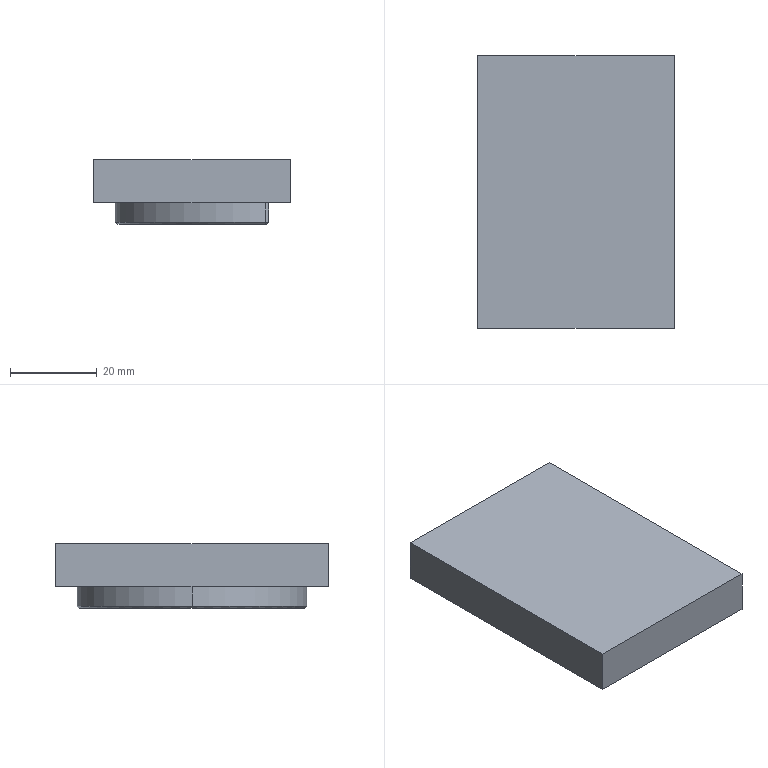NC program | NX | posted with a generic post | part box 45.394 x 63 x 15 mm
Whole program:
N10 G17 G21 G94 G90
(FLOOR_WALL_COPY , TOOL : D80)
N12 T19 M6
N14 G54
N16 G17 G0 G90 X71.5 Y0. S5000 M3
N18 G43 Z30. H19
N20 Z7.
N22 G94 G1 Z4. F1200.
N24 X66.5
N26 X-66.5
N28 X-71.5
N30 Z7.
N32 G0 Z30.
N34 X71.5
N36 Z6.
N38 G1 Z3.
N40 X66.5
N42 X-66.5
N44 X-71.5
N46 Z6.
N48 G0 Z30.
N50 X71.5
N52 Z5.
N54 G1 Z2.
N56 X66.5
N58 X-66.5
N60 X-71.5
N62 Z5.
N64 G0 Z30.
N66 X71.5
N68 Z4.
N70 G1 Z1.
N72 X66.5
N74 X-66.5
N76 X-71.5
N78 Z4.
N80 G0 Z30.
N82 X71.5
N84 Z3.
N86 G1 Z0.
N88 X66.5
N90 X-66.5
N92 X-71.5
N94 Z3.
N96 G0 Z30.
N98 M5
(HOLE_MILLING_1 , TOOL : D2)
N100 T17 M6
N102 G54
N104 G17 G0 G90 X0. Y13.197 S9500 M3
N106 G43 Z30. H17
N108 Z0.5
N110 G94 G3 X-0.253 Y12.945 R0.253 F1050.
N112 X0. Y12.692 R0.253
N114 X0. Y12.692 Z0.35 I0. J0.505
N116 X0. Y12.692 Z0.2 I0. J0.505
N118 X0. Y12.692 Z0.05 I0. J0.505
N120 X0. Y12.692 Z-0.1 I0. J0.505
N122 X0. Y12.692 Z-0.25 I0. J0.505
N124 X0. Y12.692 Z-0.4 I0. J0.505
N126 X0. Y12.692 Z-0.55 I0. J0.505
N128 X0. Y12.692 Z-0.7 I0. J0.505
N130 X0. Y12.692 Z-0.85 I0. J0.505
N132 X0. Y12.692 Z-1. I0. J0.505
N134 X0. Y12.692 Z-1.15 I0. J0.505
N136 X0. Y12.692 Z-1.3 I0. J0.505
N138 X0. Y12.692 Z-1.45 I0. J0.505
N140 X0. Y12.692 Z-1.6 I0. J0.505
N142 X0. Y12.692 Z-1.75 I0. J0.505
N144 X0. Y12.692 Z-1.9 I0. J0.505
N146 X0. Y12.692 Z-2.05 I0. J0.505
N148 X0. Y12.692 Z-2.2 I0. J0.505
N150 X0. Y12.692 Z-2.35 I0. J0.505
N152 X0. Y12.692 Z-2.5 I0. J0.505
N154 X0. Y12.692 Z-2.65 I0. J0.505
N156 X0. Y12.692 Z-2.8 I0. J0.505
N158 X0. Y12.692 Z-2.95 I0. J0.505
N160 X0. Y12.692 Z-3.1 I0. J0.505
N162 X0. Y12.692 Z-3.25 I0. J0.505
N164 X0. Y12.692 Z-3.4 I0. J0.505
N166 X0. Y12.692 Z-3.55 I0. J0.505
N168 X0. Y12.692 Z-3.7 I0. J0.505
N170 X0. Y12.692 Z-3.85 I0. J0.505
N172 X0. Y12.692 Z-4. I0. J0.505
N174 X0. Y12.692 Z-4.15 I0. J0.505
N176 X0. Y12.692 Z-4.3 I0. J0.505
N178 X0. Y12.692 Z-4.45 I0. J0.505
N180 X0. Y12.692 Z-4.6 I0. J0.505
N182 X0. Y12.692 Z-4.75 I0. J0.505
N184 X0. Y12.692 Z-4.9 I0. J0.505
N186 X-0.437 Y13.45 Z-5. R-0.505
N188 X-0.253 Y12.76 R0.505
N190 X-0.437 Y13.45 R-0.505
N192 X-0.345 Y13.105 R0.253
N194 X0. Y13.197 R0.253
N196 G0 Z30.
N198 M5
(PLANAR_PROFILE_1 , TOOL : D6A45)
N200 T01 M6
N202 G54
N204 G17 G0 G90 X-22.626 Y-9.227 S9500 M3
N206 G43 Z30. H1
N208 Z0.5
N210 G94 G1 X-22.552 Y-9.354 Z0.46 F1500.
N212 X-22.214 Y-9.553 Z0.356
N214 X-21.786 Z0.241
N216 X-21.448 Y-9.354 Z0.136
N218 X-21.25 Y-9.017 Z0.031
N220 Y-8.589 Z-0.084
N222 X-21.448 Y-8.251 Z-0.189
N224 X-21.786 Y-8.053 Z-0.294
N226 X-22.214 Z-0.408
N228 X-22.552 Y-8.251 Z-0.513
N230 X-22.75 Y-8.589 Z-0.618
N232 Y-9.017 Z-0.733
N234 X-22.552 Y-9.354 Z-0.838
N236 X-22.214 Y-9.553 Z-0.943
N238 X-22. Z-1.
N240 G3 X-21.25 Y-8.803 R0.75
N242 X-22. Y-9.553 R-0.75
N244 X-21.48 Y-9.253 R0.6
N246 G1 Z0.5
N248 G0 Z30.
N250 X-16.183 Y6.329
N252 Z0.5
N254 G1 X-16.108 Y6.202 Z0.46
N256 X-15.771 Y6.004 Z0.356
N258 X-15.342 Z0.241
N260 X-15.005 Y6.202 Z0.136
N262 X-14.806 Y6.539 Z0.031
N264 Y6.968 Z-0.084
N266 X-15.005 Y7.305 Z-0.189
N268 X-15.342 Y7.504 Z-0.294
N270 X-15.771 Z-0.408
N272 X-16.108 Y7.305 Z-0.513
N274 X-16.306 Y6.968 Z-0.618
N276 Y6.539 Z-0.733
N278 X-16.108 Y6.202 Z-0.838
N280 X-15.771 Y6.004 Z-0.943
N282 X-15.556 Z-1.
N284 G3 X-14.806 Y6.754 R0.75
N286 X-15.556 Y6.004 R-0.75
N288 X-15.037 Y6.304 R0.6
N290 G1 Z0.5
N292 G0 Z30.
N294 X23.023 Y-18.819
N296 Z0.5
N298 G1 Z-1.
N300 X23.241 Y-18.22
N302 G3 X23.136 Y-17.629 R0.6
N304 G1 X19.313 Y-13.072
N306 G2 X18.04 Y-9.391 R5.45
N308 G3 X-18.04 Y-9.391 R-18.05
N310 G2 X-19.313 Y-13.072 R5.45
N312 G1 X-23.136 Y-17.629
N314 G2 X-25.626 Y-17.146 R1.45
N316 X25.626 Y-17.146 R-26.95
N318 X23.136 Y-17.629 R1.45
N320 G3 X22.573 Y-17.424 R0.6
N322 G1 X21.777 Y-17.564
N324 Z0.5
N326 G0 Z30.
N328 X-0.028 Y13.156
N330 Z0.5
N332 G1 Z-1.
N334 X-0.52 Y12.447
N336 G3 X0. Y12.147 R0.6
N338 X1.05 Y13.197 R1.05
N340 X0. Y12.147 R-1.05
N342 X0.52 Y12.447 R0.6
N344 G1 X0.028 Y13.156
N346 Z0.5
N348 G0 Z30.
N350 X14.93 Y6.329
N352 Z0.5
N354 G1 X15.005 Y6.202 Z0.46
N356 X15.342 Y6.004 Z0.356
N358 X15.771 Z0.241
N360 X16.108 Y6.202 Z0.136
N362 X16.306 Y6.539 Z0.031
N364 Y6.968 Z-0.084
N366 X16.108 Y7.305 Z-0.189
N368 X15.771 Y7.504 Z-0.294
N370 X15.342 Z-0.408
N372 X15.005 Y7.305 Z-0.513
N374 X14.806 Y6.968 Z-0.618
N376 Y6.539 Z-0.733
N378 X15.005 Y6.202 Z-0.838
N380 X15.342 Y6.004 Z-0.943
N382 X15.556 Z-1.
N384 G3 X16.306 Y6.754 R0.75
N386 X15.556 Y6.004 R-0.75
N388 G1 X15.642 Y5.985
N390 X15.706 Y6.044
N392 Z0.5
N394 G0 Z30.
N396 X21.374 Y-9.227
N398 Z0.5
N400 G1 X21.448 Y-9.354 Z0.46
N402 X21.786 Y-9.553 Z0.356
N404 X22.214 Z0.241
N406 X22.552 Y-9.354 Z0.136
N408 X22.75 Y-9.017 Z0.031
N410 Y-8.589 Z-0.084
N412 X22.552 Y-8.251 Z-0.189
N414 X22.214 Y-8.053 Z-0.294
N416 X21.786 Z-0.408
N418 X21.448 Y-8.251 Z-0.513
N420 X21.25 Y-8.589 Z-0.618
N422 Y-9.017 Z-0.733
N424 X21.448 Y-9.354 Z-0.838
N426 X21.786 Y-9.553 Z-0.943
N428 X22. Z-1.
N430 G3 X22.75 Y-8.803 R0.75
N432 X22. Y-9.553 R-0.75
N434 X22.52 Y-9.253 R0.6
N436 G1 Z0.5
N438 G0 Z30.
N440 M5
N442 M2